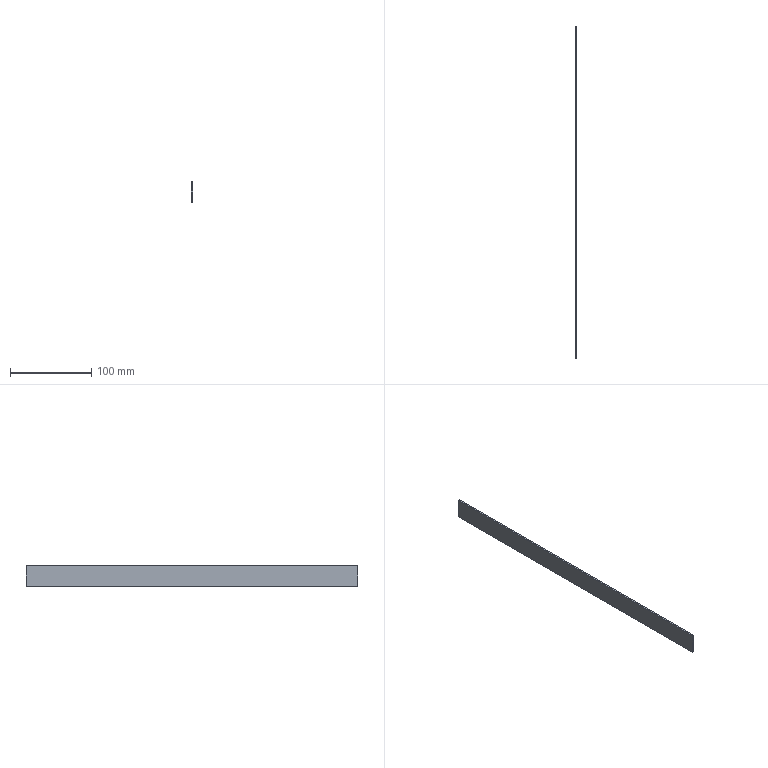Part | NX | 1 solid | 16 faces | box 2 x 409.7 x 25 mm | volume 20485 mm3 | plane 16
STEP:
#1=CARTESIAN_POINT('',(2.832,185.442,18.461));
#2=VERTEX_POINT('',#1);
#3=CARTESIAN_POINT('',(2.832,185.442,25.961));
#4=DIRECTION('',(1.,0.,0.));
#5=DIRECTION('',(0.,0.,-1.));
#6=AXIS2_PLACEMENT_3D('',#3,#4,#5);
#7=CIRCLE('',#6,7.5);
#8=EDGE_CURVE('',#2,#2,#7,.F.);
#9=ORIENTED_EDGE('',*,*,#8,.T.);
#10=EDGE_LOOP('',(#9));
#11=FACE_BOUND('',#10,.T.);
#12=CARTESIAN_POINT('',(2.832,265.442,18.461));
#13=VERTEX_POINT('',#12);
#14=CARTESIAN_POINT('',(2.832,265.442,25.961));
#15=DIRECTION('',(1.,0.,0.));
#16=DIRECTION('',(0.,0.,-1.));
#17=AXIS2_PLACEMENT_3D('',#14,#15,#16);
#18=CIRCLE('',#17,7.5);
#19=EDGE_CURVE('',#13,#13,#18,.F.);
#20=ORIENTED_EDGE('',*,*,#19,.T.);
#21=EDGE_LOOP('',(#20));
#22=FACE_BOUND('',#21,.T.);
#23=CARTESIAN_POINT('',(2.832,345.442,18.461));
#24=VERTEX_POINT('',#23);
#25=CARTESIAN_POINT('',(2.832,345.442,25.961));
#26=DIRECTION('',(1.,0.,0.));
#27=DIRECTION('',(0.,0.,-1.));
#28=AXIS2_PLACEMENT_3D('',#25,#26,#27);
#29=CIRCLE('',#28,7.5);
#30=EDGE_CURVE('',#24,#24,#29,.F.);
#31=ORIENTED_EDGE('',*,*,#30,.T.);
#32=EDGE_LOOP('',(#31));
#33=FACE_BOUND('',#32,.T.);
#34=CARTESIAN_POINT('',(2.832,425.442,18.461));
#35=VERTEX_POINT('',#34);
#36=CARTESIAN_POINT('',(2.832,425.442,25.961));
#37=DIRECTION('',(1.,0.,0.));
#38=DIRECTION('',(0.,0.,-1.));
#39=AXIS2_PLACEMENT_3D('',#36,#37,#38);
#40=CIRCLE('',#39,7.5);
#41=EDGE_CURVE('',#35,#35,#40,.F.);
#42=ORIENTED_EDGE('',*,*,#41,.T.);
#43=EDGE_LOOP('',(#42));
#44=FACE_BOUND('',#43,.T.);
#45=CARTESIAN_POINT('',(2.832,505.442,18.461));
#46=VERTEX_POINT('',#45);
#47=CARTESIAN_POINT('',(2.832,505.442,25.961));
#48=DIRECTION('',(1.,0.,0.));
#49=DIRECTION('',(0.,0.,-1.));
#50=AXIS2_PLACEMENT_3D('',#47,#48,#49);
#51=CIRCLE('',#50,7.5);
#52=EDGE_CURVE('',#46,#46,#51,.F.);
#53=ORIENTED_EDGE('',*,*,#52,.T.);
#54=EDGE_LOOP('',(#53));
#55=FACE_BOUND('',#54,.T.);
#56=CARTESIAN_POINT('',(2.832,120.592,38.461));
#57=VERTEX_POINT('',#56);
#58=CARTESIAN_POINT('',(2.832,530.292,38.461));
#59=VERTEX_POINT('',#58);
#60=CARTESIAN_POINT('',(2.832,120.592,38.461));
#61=DIRECTION('',(0.,1.,0.));
#62=VECTOR('',#61,1000.);
#63=LINE('',#60,#62);
#64=EDGE_CURVE('',#57,#59,#63,.T.);
#65=ORIENTED_EDGE('',*,*,#64,.F.);
#66=CARTESIAN_POINT('',(2.832,120.592,13.461));
#67=VERTEX_POINT('',#66);
#68=CARTESIAN_POINT('',(2.832,120.592,25.961));
#69=DIRECTION('',(0.,0.,-1.));
#70=VECTOR('',#69,1000.);
#71=LINE('',#68,#70);
#72=EDGE_CURVE('',#67,#57,#71,.F.);
#73=ORIENTED_EDGE('',*,*,#72,.F.);
#74=CARTESIAN_POINT('',(2.832,530.292,13.461));
#75=VERTEX_POINT('',#74);
#76=CARTESIAN_POINT('',(2.832,120.592,13.461));
#77=DIRECTION('',(0.,1.,0.));
#78=VECTOR('',#77,1000.);
#79=LINE('',#76,#78);
#80=EDGE_CURVE('',#75,#67,#79,.F.);
#81=ORIENTED_EDGE('',*,*,#80,.F.);
#82=CARTESIAN_POINT('',(2.832,530.292,25.961));
#83=DIRECTION('',(0.,0.,1.));
#84=VECTOR('',#83,1000.);
#85=LINE('',#82,#84);
#86=EDGE_CURVE('',#59,#75,#85,.F.);
#87=ORIENTED_EDGE('',*,*,#86,.F.);
#88=EDGE_LOOP('',(#65,#73,#81,#87));
#89=FACE_BOUND('',#88,.T.);
#90=CARTESIAN_POINT('',(2.832,465.442,18.461));
#91=VERTEX_POINT('',#90);
#92=CARTESIAN_POINT('',(2.832,465.442,25.961));
#93=DIRECTION('',(1.,0.,0.));
#94=DIRECTION('',(0.,0.,-1.));
#95=AXIS2_PLACEMENT_3D('',#92,#93,#94);
#96=CIRCLE('',#95,7.5);
#97=EDGE_CURVE('',#91,#91,#96,.F.);
#98=ORIENTED_EDGE('',*,*,#97,.T.);
#99=EDGE_LOOP('',(#98));
#100=FACE_BOUND('',#99,.T.);
#101=CARTESIAN_POINT('',(2.832,385.442,18.461));
#102=VERTEX_POINT('',#101);
#103=CARTESIAN_POINT('',(2.832,385.442,25.961));
#104=DIRECTION('',(1.,0.,0.));
#105=DIRECTION('',(0.,0.,-1.));
#106=AXIS2_PLACEMENT_3D('',#103,#104,#105);
#107=CIRCLE('',#106,7.5);
#108=EDGE_CURVE('',#102,#102,#107,.F.);
#109=ORIENTED_EDGE('',*,*,#108,.T.);
#110=EDGE_LOOP('',(#109));
#111=FACE_BOUND('',#110,.T.);
#112=CARTESIAN_POINT('',(2.832,305.442,18.461));
#113=VERTEX_POINT('',#112);
#114=CARTESIAN_POINT('',(2.832,305.442,25.961));
#115=DIRECTION('',(1.,0.,0.));
#116=DIRECTION('',(0.,0.,-1.));
#117=AXIS2_PLACEMENT_3D('',#114,#115,#116);
#118=CIRCLE('',#117,7.5);
#119=EDGE_CURVE('',#113,#113,#118,.F.);
#120=ORIENTED_EDGE('',*,*,#119,.T.);
#121=EDGE_LOOP('',(#120));
#122=FACE_BOUND('',#121,.T.);
#123=CARTESIAN_POINT('',(2.832,225.442,18.461));
#124=VERTEX_POINT('',#123);
#125=CARTESIAN_POINT('',(2.832,225.442,25.961));
#126=DIRECTION('',(1.,0.,0.));
#127=DIRECTION('',(0.,0.,-1.));
#128=AXIS2_PLACEMENT_3D('',#125,#126,#127);
#129=CIRCLE('',#128,7.5);
#130=EDGE_CURVE('',#124,#124,#129,.F.);
#131=ORIENTED_EDGE('',*,*,#130,.T.);
#132=EDGE_LOOP('',(#131));
#133=FACE_BOUND('',#132,.T.);
#134=CARTESIAN_POINT('',(2.832,145.442,18.461));
#135=VERTEX_POINT('',#134);
#136=CARTESIAN_POINT('',(2.832,145.442,25.961));
#137=DIRECTION('',(1.,0.,0.));
#138=DIRECTION('',(0.,0.,-1.));
#139=AXIS2_PLACEMENT_3D('',#136,#137,#138);
#140=CIRCLE('',#139,7.5);
#141=EDGE_CURVE('',#135,#135,#140,.F.);
#142=ORIENTED_EDGE('',*,*,#141,.T.);
#143=EDGE_LOOP('',(#142));
#144=FACE_BOUND('',#143,.T.);
#145=CARTESIAN_POINT('',(2.832,120.592,13.461));
#146=DIRECTION('',(1.,0.,0.));
#147=DIRECTION('',(0.,0.,-1.));
#148=AXIS2_PLACEMENT_3D('',#145,#146,#147);
#149=PLANE('',#148);
#150=ADVANCED_FACE('',(#11,#22,#33,#44,#55,#89,#100,#111,#122,#133,#144),#149,.T.);
#151=ORIENTED_EDGE('',*,*,#141,.F.);
#152=EDGE_LOOP('',(#151));
#153=FACE_BOUND('',#152,.T.);
#154=CARTESIAN_POINT('',(2.832,120.592,13.461));
#155=DIRECTION('',(1.,0.,0.));
#156=DIRECTION('',(0.,0.,-1.));
#157=AXIS2_PLACEMENT_3D('',#154,#155,#156);
#158=PLANE('',#157);
#159=ADVANCED_FACE('',(#153),#158,.T.);
#160=ORIENTED_EDGE('',*,*,#8,.F.);
#161=EDGE_LOOP('',(#160));
#162=FACE_BOUND('',#161,.T.);
#163=CARTESIAN_POINT('',(2.832,120.592,13.461));
#164=DIRECTION('',(1.,0.,0.));
#165=DIRECTION('',(0.,0.,-1.));
#166=AXIS2_PLACEMENT_3D('',#163,#164,#165);
#167=PLANE('',#166);
#168=ADVANCED_FACE('',(#162),#167,.T.);
#169=ORIENTED_EDGE('',*,*,#130,.F.);
#170=EDGE_LOOP('',(#169));
#171=FACE_BOUND('',#170,.T.);
#172=CARTESIAN_POINT('',(2.832,120.592,13.461));
#173=DIRECTION('',(1.,0.,0.));
#174=DIRECTION('',(0.,0.,-1.));
#175=AXIS2_PLACEMENT_3D('',#172,#173,#174);
#176=PLANE('',#175);
#177=ADVANCED_FACE('',(#171),#176,.T.);
#178=ORIENTED_EDGE('',*,*,#19,.F.);
#179=EDGE_LOOP('',(#178));
#180=FACE_BOUND('',#179,.T.);
#181=CARTESIAN_POINT('',(2.832,120.592,13.461));
#182=DIRECTION('',(1.,0.,0.));
#183=DIRECTION('',(0.,0.,-1.));
#184=AXIS2_PLACEMENT_3D('',#181,#182,#183);
#185=PLANE('',#184);
#186=ADVANCED_FACE('',(#180),#185,.T.);
#187=ORIENTED_EDGE('',*,*,#119,.F.);
#188=EDGE_LOOP('',(#187));
#189=FACE_BOUND('',#188,.T.);
#190=CARTESIAN_POINT('',(2.832,120.592,13.461));
#191=DIRECTION('',(1.,0.,0.));
#192=DIRECTION('',(0.,0.,-1.));
#193=AXIS2_PLACEMENT_3D('',#190,#191,#192);
#194=PLANE('',#193);
#195=ADVANCED_FACE('',(#189),#194,.T.);
#196=ORIENTED_EDGE('',*,*,#30,.F.);
#197=EDGE_LOOP('',(#196));
#198=FACE_BOUND('',#197,.T.);
#199=CARTESIAN_POINT('',(2.832,120.592,13.461));
#200=DIRECTION('',(1.,0.,0.));
#201=DIRECTION('',(0.,0.,-1.));
#202=AXIS2_PLACEMENT_3D('',#199,#200,#201);
#203=PLANE('',#202);
#204=ADVANCED_FACE('',(#198),#203,.T.);
#205=ORIENTED_EDGE('',*,*,#108,.F.);
#206=EDGE_LOOP('',(#205));
#207=FACE_BOUND('',#206,.T.);
#208=CARTESIAN_POINT('',(2.832,120.592,13.461));
#209=DIRECTION('',(1.,0.,0.));
#210=DIRECTION('',(0.,0.,-1.));
#211=AXIS2_PLACEMENT_3D('',#208,#209,#210);
#212=PLANE('',#211);
#213=ADVANCED_FACE('',(#207),#212,.T.);
#214=ORIENTED_EDGE('',*,*,#41,.F.);
#215=EDGE_LOOP('',(#214));
#216=FACE_BOUND('',#215,.T.);
#217=CARTESIAN_POINT('',(2.832,120.592,13.461));
#218=DIRECTION('',(1.,0.,0.));
#219=DIRECTION('',(0.,0.,-1.));
#220=AXIS2_PLACEMENT_3D('',#217,#218,#219);
#221=PLANE('',#220);
#222=ADVANCED_FACE('',(#216),#221,.T.);
#223=ORIENTED_EDGE('',*,*,#97,.F.);
#224=EDGE_LOOP('',(#223));
#225=FACE_BOUND('',#224,.T.);
#226=CARTESIAN_POINT('',(2.832,120.592,13.461));
#227=DIRECTION('',(1.,0.,0.));
#228=DIRECTION('',(0.,0.,-1.));
#229=AXIS2_PLACEMENT_3D('',#226,#227,#228);
#230=PLANE('',#229);
#231=ADVANCED_FACE('',(#225),#230,.T.);
#232=CARTESIAN_POINT('',(0.8318,530.292,13.461));
#233=VERTEX_POINT('',#232);
#234=CARTESIAN_POINT('',(0.8318,120.592,13.461));
#235=VERTEX_POINT('',#234);
#236=CARTESIAN_POINT('',(0.8318,120.592,13.461));
#237=DIRECTION('',(0.,1.,0.));
#238=VECTOR('',#237,1000.);
#239=LINE('',#236,#238);
#240=EDGE_CURVE('',#233,#235,#239,.F.);
#241=ORIENTED_EDGE('',*,*,#240,.T.);
#242=CARTESIAN_POINT('',(0.8318,120.592,38.461));
#243=VERTEX_POINT('',#242);
#244=CARTESIAN_POINT('',(0.8318,120.592,38.461));
#245=DIRECTION('',(0.,0.,1.));
#246=VECTOR('',#245,1000.);
#247=LINE('',#244,#246);
#248=EDGE_CURVE('',#235,#243,#247,.T.);
#249=ORIENTED_EDGE('',*,*,#248,.T.);
#250=CARTESIAN_POINT('',(0.8318,530.292,38.461));
#251=VERTEX_POINT('',#250);
#252=CARTESIAN_POINT('',(0.8318,120.592,38.461));
#253=DIRECTION('',(0.,1.,0.));
#254=VECTOR('',#253,1000.);
#255=LINE('',#252,#254);
#256=EDGE_CURVE('',#243,#251,#255,.T.);
#257=ORIENTED_EDGE('',*,*,#256,.T.);
#258=CARTESIAN_POINT('',(0.8318,530.292,38.461));
#259=DIRECTION('',(0.,0.,1.));
#260=VECTOR('',#259,1000.);
#261=LINE('',#258,#260);
#262=EDGE_CURVE('',#251,#233,#261,.F.);
#263=ORIENTED_EDGE('',*,*,#262,.T.);
#264=EDGE_LOOP('',(#241,#249,#257,#263));
#265=FACE_BOUND('',#264,.T.);
#266=CARTESIAN_POINT('',(0.8318,120.592,38.461));
#267=DIRECTION('',(-1.,0.,0.));
#268=DIRECTION('',(0.,0.,1.));
#269=AXIS2_PLACEMENT_3D('',#266,#267,#268);
#270=PLANE('',#269);
#271=ADVANCED_FACE('',(#265),#270,.T.);
#272=CARTESIAN_POINT('',(-13.568,120.592,38.461));
#273=DIRECTION('',(1.,0.,0.));
#274=VECTOR('',#273,1000.);
#275=LINE('',#272,#274);
#276=EDGE_CURVE('',#57,#243,#275,.F.);
#277=ORIENTED_EDGE('',*,*,#276,.T.);
#278=ORIENTED_EDGE('',*,*,#248,.F.);
#279=CARTESIAN_POINT('',(-13.568,120.592,13.461));
#280=DIRECTION('',(1.,0.,0.));
#281=VECTOR('',#280,1000.);
#282=LINE('',#279,#281);
#283=EDGE_CURVE('',#235,#67,#282,.T.);
#284=ORIENTED_EDGE('',*,*,#283,.T.);
#285=ORIENTED_EDGE('',*,*,#72,.T.);
#286=EDGE_LOOP('',(#277,#278,#284,#285));
#287=FACE_BOUND('',#286,.T.);
#288=CARTESIAN_POINT('',(-13.568,120.592,25.961));
#289=DIRECTION('',(0.,-1.,0.));
#290=DIRECTION('',(0.,0.,-1.));
#291=AXIS2_PLACEMENT_3D('',#288,#289,#290);
#292=PLANE('',#291);
#293=ADVANCED_FACE('',(#287),#292,.T.);
#294=ORIENTED_EDGE('',*,*,#80,.T.);
#295=ORIENTED_EDGE('',*,*,#283,.F.);
#296=ORIENTED_EDGE('',*,*,#240,.F.);
#297=CARTESIAN_POINT('',(0.8318,530.292,13.461));
#298=DIRECTION('',(-1.,0.,0.));
#299=VECTOR('',#298,1000.);
#300=LINE('',#297,#299);
#301=EDGE_CURVE('',#233,#75,#300,.F.);
#302=ORIENTED_EDGE('',*,*,#301,.T.);
#303=EDGE_LOOP('',(#294,#295,#296,#302));
#304=FACE_BOUND('',#303,.T.);
#305=CARTESIAN_POINT('',(0.8318,120.592,13.461));
#306=DIRECTION('',(0.,0.,-1.));
#307=DIRECTION('',(-1.,0.,0.));
#308=AXIS2_PLACEMENT_3D('',#305,#306,#307);
#309=PLANE('',#308);
#310=ADVANCED_FACE('',(#304),#309,.T.);
#311=ORIENTED_EDGE('',*,*,#301,.F.);
#312=ORIENTED_EDGE('',*,*,#262,.F.);
#313=CARTESIAN_POINT('',(-13.568,530.292,38.461));
#314=DIRECTION('',(1.,0.,0.));
#315=VECTOR('',#314,1000.);
#316=LINE('',#313,#315);
#317=EDGE_CURVE('',#251,#59,#316,.T.);
#318=ORIENTED_EDGE('',*,*,#317,.T.);
#319=ORIENTED_EDGE('',*,*,#86,.T.);
#320=EDGE_LOOP('',(#311,#312,#318,#319));
#321=FACE_BOUND('',#320,.T.);
#322=CARTESIAN_POINT('',(-13.568,530.292,25.961));
#323=DIRECTION('',(0.,1.,0.));
#324=DIRECTION('',(0.,0.,1.));
#325=AXIS2_PLACEMENT_3D('',#322,#323,#324);
#326=PLANE('',#325);
#327=ADVANCED_FACE('',(#321),#326,.T.);
#328=ORIENTED_EDGE('',*,*,#256,.F.);
#329=ORIENTED_EDGE('',*,*,#276,.F.);
#330=ORIENTED_EDGE('',*,*,#64,.T.);
#331=ORIENTED_EDGE('',*,*,#317,.F.);
#332=EDGE_LOOP('',(#328,#329,#330,#331));
#333=FACE_BOUND('',#332,.T.);
#334=CARTESIAN_POINT('',(2.832,120.592,38.461));
#335=DIRECTION('',(0.,0.,1.));
#336=DIRECTION('',(1.,0.,0.));
#337=AXIS2_PLACEMENT_3D('',#334,#335,#336);
#338=PLANE('',#337);
#339=ADVANCED_FACE('',(#333),#338,.T.);
#340=ORIENTED_EDGE('',*,*,#52,.F.);
#341=EDGE_LOOP('',(#340));
#342=FACE_BOUND('',#341,.T.);
#343=CARTESIAN_POINT('',(2.832,120.592,13.461));
#344=DIRECTION('',(1.,0.,0.));
#345=DIRECTION('',(0.,0.,-1.));
#346=AXIS2_PLACEMENT_3D('',#343,#344,#345);
#347=PLANE('',#346);
#348=ADVANCED_FACE('',(#342),#347,.T.);
#349=CLOSED_SHELL('',(#150,#159,#168,#177,#186,#195,#204,#213,#222,#231,#271,#293,#310,#327,#339,#348));
#350=MANIFOLD_SOLID_BREP('',#349);
#351=(LENGTH_UNIT()NAMED_UNIT(*)SI_UNIT(.MILLI.,.METRE.));
#352=UNCERTAINTY_MEASURE_WITH_UNIT(LENGTH_MEASURE(0.00001),#351,'','');
#353=(NAMED_UNIT(*)PLANE_ANGLE_UNIT()SI_UNIT($,.RADIAN.));
#354=(NAMED_UNIT(*)SI_UNIT($,.STERADIAN.)SOLID_ANGLE_UNIT());
#355=(GEOMETRIC_REPRESENTATION_CONTEXT(3)GLOBAL_UNCERTAINTY_ASSIGNED_CONTEXT((#352))GLOBAL_UNIT_ASSIGNED_CONTEXT((#351,#353,#354))REPRESENTATION_CONTEXT('',''));
#356=ADVANCED_BREP_SHAPE_REPRESENTATION('',(#350),#355);